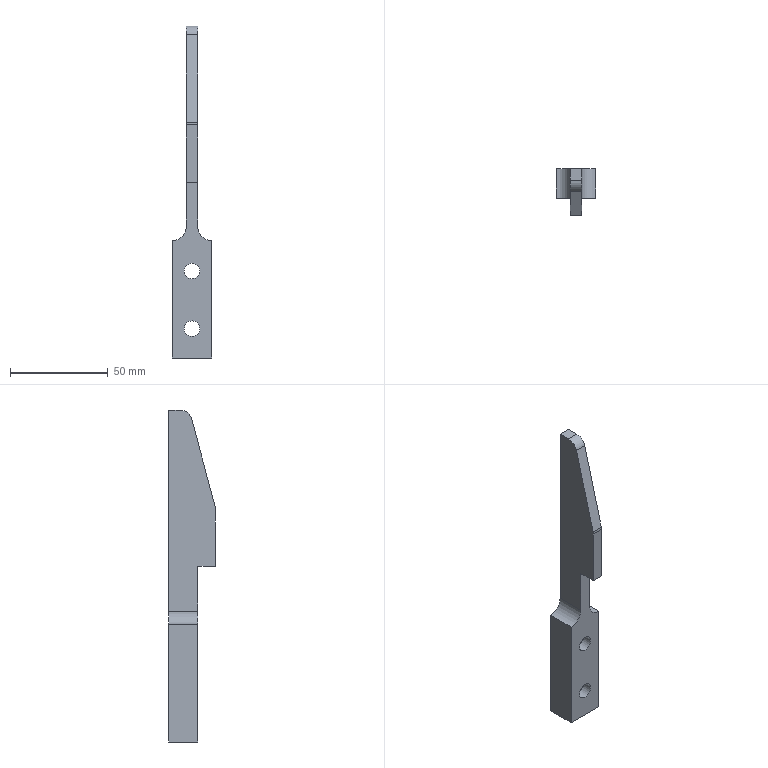Part | NX | features solid 2 | 1 solid | 21 faces | box 20 x 24 x 170 mm | volume 26920 mm3 | plane 13 | cylinder 8 | commonest cylinder face diameters 14 x4 8 x2 10 x1 12 x1
STEP:
#1=CARTESIAN_POINT('',(-125.,490.,-140.));
#2=VERTEX_POINT('',#1);
#3=CARTESIAN_POINT('',(-125.,490.,-80.));
#4=VERTEX_POINT('',#3);
#5=CARTESIAN_POINT('',(-125.,490.,-110.));
#6=DIRECTION('',(0.,0.,1.));
#7=VECTOR('',#6,1000.);
#8=LINE('',#5,#7);
#9=EDGE_CURVE('',#2,#4,#8,.T.);
#10=ORIENTED_EDGE('',*,*,#9,.F.);
#11=CARTESIAN_POINT('',(-125.,505.,-140.));
#12=VERTEX_POINT('',#11);
#13=CARTESIAN_POINT('',(-125.,490.,-140.));
#14=DIRECTION('',(0.,1.,0.));
#15=VECTOR('',#14,1000.);
#16=LINE('',#13,#15);
#17=EDGE_CURVE('',#2,#12,#16,.T.);
#18=ORIENTED_EDGE('',*,*,#17,.T.);
#19=CARTESIAN_POINT('',(-125.,505.,-80.));
#20=VERTEX_POINT('',#19);
#21=CARTESIAN_POINT('',(-125.,505.,-110.));
#22=DIRECTION('',(0.,0.,1.));
#23=VECTOR('',#22,1000.);
#24=LINE('',#21,#23);
#25=EDGE_CURVE('',#12,#20,#24,.T.);
#26=ORIENTED_EDGE('',*,*,#25,.T.);
#27=CARTESIAN_POINT('',(-125.,490.,-80.));
#28=DIRECTION('',(0.,1.,0.));
#29=VECTOR('',#28,1000.);
#30=LINE('',#27,#29);
#31=EDGE_CURVE('',#4,#20,#30,.T.);
#32=ORIENTED_EDGE('',*,*,#31,.F.);
#33=EDGE_LOOP('',(#10,#18,#26,#32));
#34=FACE_BOUND('',#33,.T.);
#35=CARTESIAN_POINT('',(-125.,490.,-110.));
#36=DIRECTION('',(1.,0.,0.));
#37=DIRECTION('',(0.,1.,0.));
#38=AXIS2_PLACEMENT_3D('',#35,#36,#37);
#39=PLANE('',#38);
#40=ADVANCED_FACE('',(#34),#39,.T.);
#41=CARTESIAN_POINT('',(-135.,505.,-118.));
#42=VERTEX_POINT('',#41);
#43=CARTESIAN_POINT('',(-135.,505.,-125.));
#44=DIRECTION('',(0.,-1.,0.));
#45=DIRECTION('',(0.,0.,1.));
#46=AXIS2_PLACEMENT_3D('',#43,#44,#45);
#47=CIRCLE('',#46,7.);
#48=EDGE_CURVE('',#42,#42,#47,.T.);
#49=ORIENTED_EDGE('',*,*,#48,.T.);
#50=EDGE_LOOP('',(#49));
#51=FACE_BOUND('',#50,.T.);
#52=CARTESIAN_POINT('',(-135.,505.,-102.5));
#53=VERTEX_POINT('',#52);
#54=CARTESIAN_POINT('',(-135.,505.,-95.5));
#55=DIRECTION('',(0.,1.,0.));
#56=DIRECTION('',(0.,0.,-1.));
#57=AXIS2_PLACEMENT_3D('',#54,#55,#56);
#58=CIRCLE('',#57,7.);
#59=EDGE_CURVE('',#53,#53,#58,.F.);
#60=ORIENTED_EDGE('',*,*,#59,.T.);
#61=EDGE_LOOP('',(#60));
#62=FACE_BOUND('',#61,.T.);
#63=ORIENTED_EDGE('',*,*,#25,.F.);
#64=CARTESIAN_POINT('',(-145.,505.,-140.));
#65=VERTEX_POINT('',#64);
#66=CARTESIAN_POINT('',(-125.,505.,-140.));
#67=DIRECTION('',(-1.,0.,0.));
#68=VECTOR('',#67,1000.);
#69=LINE('',#66,#68);
#70=EDGE_CURVE('',#12,#65,#69,.T.);
#71=ORIENTED_EDGE('',*,*,#70,.T.);
#72=CARTESIAN_POINT('',(-145.,505.,-80.));
#73=VERTEX_POINT('',#72);
#74=CARTESIAN_POINT('',(-145.,505.,-110.));
#75=DIRECTION('',(0.,0.,1.));
#76=VECTOR('',#75,1000.);
#77=LINE('',#74,#76);
#78=EDGE_CURVE('',#65,#73,#77,.T.);
#79=ORIENTED_EDGE('',*,*,#78,.T.);
#80=CARTESIAN_POINT('',(-138.,505.,-73.));
#81=VERTEX_POINT('',#80);
#82=CARTESIAN_POINT('',(-145.,505.,-73.));
#83=DIRECTION('',(0.,1.,0.));
#84=DIRECTION('',(0.,0.,-1.));
#85=AXIS2_PLACEMENT_3D('',#82,#83,#84);
#86=CIRCLE('',#85,7.);
#87=EDGE_CURVE('',#73,#81,#86,.F.);
#88=ORIENTED_EDGE('',*,*,#87,.T.);
#89=CARTESIAN_POINT('',(-138.,505.,30.));
#90=VERTEX_POINT('',#89);
#91=CARTESIAN_POINT('',(-138.,505.,-50.));
#92=DIRECTION('',(0.,0.,1.));
#93=VECTOR('',#92,1000.);
#94=LINE('',#91,#93);
#95=EDGE_CURVE('',#81,#90,#94,.T.);
#96=ORIENTED_EDGE('',*,*,#95,.T.);
#97=CARTESIAN_POINT('',(-132.,505.,30.));
#98=VERTEX_POINT('',#97);
#99=CARTESIAN_POINT('',(-132.,505.,30.));
#100=DIRECTION('',(-1.,0.,0.));
#101=VECTOR('',#100,1000.);
#102=LINE('',#99,#101);
#103=EDGE_CURVE('',#98,#90,#102,.T.);
#104=ORIENTED_EDGE('',*,*,#103,.F.);
#105=CARTESIAN_POINT('',(-132.,505.,-73.));
#106=VERTEX_POINT('',#105);
#107=CARTESIAN_POINT('',(-132.,505.,-50.));
#108=DIRECTION('',(0.,0.,1.));
#109=VECTOR('',#108,1000.);
#110=LINE('',#107,#109);
#111=EDGE_CURVE('',#106,#98,#110,.T.);
#112=ORIENTED_EDGE('',*,*,#111,.F.);
#113=CARTESIAN_POINT('',(-125.,505.,-73.));
#114=DIRECTION('',(0.,1.,0.));
#115=DIRECTION('',(0.,0.,-1.));
#116=AXIS2_PLACEMENT_3D('',#113,#114,#115);
#117=CIRCLE('',#116,7.);
#118=EDGE_CURVE('',#106,#20,#117,.F.);
#119=ORIENTED_EDGE('',*,*,#118,.T.);
#120=EDGE_LOOP('',(#63,#71,#79,#88,#96,#104,#112,#119));
#121=FACE_BOUND('',#120,.T.);
#122=CARTESIAN_POINT('',(-125.,505.,-110.));
#123=DIRECTION('',(0.,1.,0.));
#124=DIRECTION('',(-1.,0.,0.));
#125=AXIS2_PLACEMENT_3D('',#122,#123,#124);
#126=PLANE('',#125);
#127=ADVANCED_FACE('',(#51,#62,#121),#126,.T.);
#128=ORIENTED_EDGE('',*,*,#78,.F.);
#129=CARTESIAN_POINT('',(-145.,490.,-140.));
#130=VERTEX_POINT('',#129);
#131=CARTESIAN_POINT('',(-145.,490.,-140.));
#132=DIRECTION('',(0.,1.,0.));
#133=VECTOR('',#132,1000.);
#134=LINE('',#131,#133);
#135=EDGE_CURVE('',#130,#65,#134,.T.);
#136=ORIENTED_EDGE('',*,*,#135,.F.);
#137=CARTESIAN_POINT('',(-145.,490.,-80.));
#138=VERTEX_POINT('',#137);
#139=CARTESIAN_POINT('',(-145.,490.,-110.));
#140=DIRECTION('',(0.,0.,1.));
#141=VECTOR('',#140,1000.);
#142=LINE('',#139,#141);
#143=EDGE_CURVE('',#130,#138,#142,.T.);
#144=ORIENTED_EDGE('',*,*,#143,.T.);
#145=CARTESIAN_POINT('',(-145.,490.,-80.));
#146=DIRECTION('',(0.,1.,0.));
#147=VECTOR('',#146,1000.);
#148=LINE('',#145,#147);
#149=EDGE_CURVE('',#138,#73,#148,.T.);
#150=ORIENTED_EDGE('',*,*,#149,.T.);
#151=EDGE_LOOP('',(#128,#136,#144,#150));
#152=FACE_BOUND('',#151,.T.);
#153=CARTESIAN_POINT('',(-145.,490.,-110.));
#154=DIRECTION('',(1.,0.,0.));
#155=DIRECTION('',(0.,1.,0.));
#156=AXIS2_PLACEMENT_3D('',#153,#154,#155);
#157=PLANE('',#156);
#158=ADVANCED_FACE('',(#152),#157,.F.);
#159=CARTESIAN_POINT('',(-135.,490.,-99.5));
#160=VERTEX_POINT('',#159);
#161=CARTESIAN_POINT('',(-135.,490.,-95.5));
#162=DIRECTION('',(0.,1.,0.));
#163=DIRECTION('',(0.,0.,-1.));
#164=AXIS2_PLACEMENT_3D('',#161,#162,#163);
#165=CIRCLE('',#164,4.);
#166=EDGE_CURVE('',#160,#160,#165,.T.);
#167=ORIENTED_EDGE('',*,*,#166,.T.);
#168=EDGE_LOOP('',(#167));
#169=FACE_BOUND('',#168,.T.);
#170=CARTESIAN_POINT('',(-135.,490.,-129.));
#171=VERTEX_POINT('',#170);
#172=CARTESIAN_POINT('',(-135.,490.,-125.));
#173=DIRECTION('',(0.,1.,0.));
#174=DIRECTION('',(0.,0.,-1.));
#175=AXIS2_PLACEMENT_3D('',#172,#173,#174);
#176=CIRCLE('',#175,4.);
#177=EDGE_CURVE('',#171,#171,#176,.T.);
#178=ORIENTED_EDGE('',*,*,#177,.T.);
#179=EDGE_LOOP('',(#178));
#180=FACE_BOUND('',#179,.T.);
#181=CARTESIAN_POINT('',(-132.,490.,-50.));
#182=VERTEX_POINT('',#181);
#183=CARTESIAN_POINT('',(-132.,490.,-73.));
#184=VERTEX_POINT('',#183);
#185=CARTESIAN_POINT('',(-132.,490.,-43.));
#186=DIRECTION('',(0.,0.,1.));
#187=VECTOR('',#186,1000.);
#188=LINE('',#185,#187);
#189=EDGE_CURVE('',#182,#184,#188,.F.);
#190=ORIENTED_EDGE('',*,*,#189,.F.);
#191=CARTESIAN_POINT('',(-138.,490.,-50.));
#192=VERTEX_POINT('',#191);
#193=CARTESIAN_POINT('',(-132.,490.,-50.));
#194=DIRECTION('',(1.,0.,0.));
#195=VECTOR('',#194,1000.);
#196=LINE('',#193,#195);
#197=EDGE_CURVE('',#182,#192,#196,.F.);
#198=ORIENTED_EDGE('',*,*,#197,.T.);
#199=CARTESIAN_POINT('',(-138.,490.,-73.));
#200=VERTEX_POINT('',#199);
#201=CARTESIAN_POINT('',(-138.,490.,-43.));
#202=DIRECTION('',(0.,0.,-1.));
#203=VECTOR('',#202,1000.);
#204=LINE('',#201,#203);
#205=EDGE_CURVE('',#192,#200,#204,.T.);
#206=ORIENTED_EDGE('',*,*,#205,.T.);
#207=CARTESIAN_POINT('',(-145.,490.,-73.));
#208=DIRECTION('',(0.,1.,0.));
#209=DIRECTION('',(0.,0.,-1.));
#210=AXIS2_PLACEMENT_3D('',#207,#208,#209);
#211=CIRCLE('',#210,7.);
#212=EDGE_CURVE('',#200,#138,#211,.T.);
#213=ORIENTED_EDGE('',*,*,#212,.T.);
#214=ORIENTED_EDGE('',*,*,#143,.F.);
#215=CARTESIAN_POINT('',(-125.,490.,-140.));
#216=DIRECTION('',(-1.,0.,0.));
#217=VECTOR('',#216,1000.);
#218=LINE('',#215,#217);
#219=EDGE_CURVE('',#2,#130,#218,.T.);
#220=ORIENTED_EDGE('',*,*,#219,.F.);
#221=ORIENTED_EDGE('',*,*,#9,.T.);
#222=CARTESIAN_POINT('',(-125.,490.,-73.));
#223=DIRECTION('',(0.,1.,0.));
#224=DIRECTION('',(0.,0.,-1.));
#225=AXIS2_PLACEMENT_3D('',#222,#223,#224);
#226=CIRCLE('',#225,7.);
#227=EDGE_CURVE('',#4,#184,#226,.T.);
#228=ORIENTED_EDGE('',*,*,#227,.T.);
#229=EDGE_LOOP('',(#190,#198,#206,#213,#214,#220,#221,#228));
#230=FACE_BOUND('',#229,.T.);
#231=CARTESIAN_POINT('',(-125.,490.,-110.));
#232=DIRECTION('',(0.,1.,0.));
#233=DIRECTION('',(-1.,0.,0.));
#234=AXIS2_PLACEMENT_3D('',#231,#232,#233);
#235=PLANE('',#234);
#236=ADVANCED_FACE('',(#169,#180,#230),#235,.F.);
#237=ORIENTED_EDGE('',*,*,#135,.T.);
#238=ORIENTED_EDGE('',*,*,#70,.F.);
#239=ORIENTED_EDGE('',*,*,#17,.F.);
#240=ORIENTED_EDGE('',*,*,#219,.T.);
#241=EDGE_LOOP('',(#237,#238,#239,#240));
#242=FACE_BOUND('',#241,.T.);
#243=CARTESIAN_POINT('',(-125.,490.,-140.));
#244=DIRECTION('',(0.,0.,1.));
#245=DIRECTION('',(0.,1.,0.));
#246=AXIS2_PLACEMENT_3D('',#243,#244,#245);
#247=PLANE('',#246);
#248=ADVANCED_FACE('',(#242),#247,.F.);
#249=CARTESIAN_POINT('',(-132.,493.206,25.553));
#250=VERTEX_POINT('',#249);
#251=CARTESIAN_POINT('',(-132.,481.17,-19.364));
#252=VERTEX_POINT('',#251);
#253=CARTESIAN_POINT('',(-132.,478.398,-29.711));
#254=DIRECTION('',(0.,-0.2588,-0.9659));
#255=VECTOR('',#254,1000.);
#256=LINE('',#253,#255);
#257=EDGE_CURVE('',#250,#252,#256,.T.);
#258=ORIENTED_EDGE('',*,*,#257,.T.);
#259=CARTESIAN_POINT('',(-132.,481.,-20.658));
#260=VERTEX_POINT('',#259);
#261=CARTESIAN_POINT('',(-132.,486.,-20.658));
#262=DIRECTION('',(1.,0.,0.));
#263=DIRECTION('',(0.,0.,-1.));
#264=AXIS2_PLACEMENT_3D('',#261,#262,#263);
#265=CIRCLE('',#264,5.);
#266=EDGE_CURVE('',#252,#260,#265,.T.);
#267=ORIENTED_EDGE('',*,*,#266,.T.);
#268=CARTESIAN_POINT('',(-132.,481.,-50.));
#269=VERTEX_POINT('',#268);
#270=CARTESIAN_POINT('',(-132.,481.,-43.));
#271=DIRECTION('',(0.,0.,1.));
#272=VECTOR('',#271,1000.);
#273=LINE('',#270,#272);
#274=EDGE_CURVE('',#269,#260,#273,.T.);
#275=ORIENTED_EDGE('',*,*,#274,.F.);
#276=CARTESIAN_POINT('',(-132.,490.,-50.));
#277=DIRECTION('',(0.,1.,0.));
#278=VECTOR('',#277,1000.);
#279=LINE('',#276,#278);
#280=EDGE_CURVE('',#182,#269,#279,.F.);
#281=ORIENTED_EDGE('',*,*,#280,.F.);
#282=ORIENTED_EDGE('',*,*,#189,.T.);
#283=CARTESIAN_POINT('',(-132.,505.,-73.));
#284=DIRECTION('',(0.,1.,0.));
#285=VECTOR('',#284,1000.);
#286=LINE('',#283,#285);
#287=EDGE_CURVE('',#184,#106,#286,.T.);
#288=ORIENTED_EDGE('',*,*,#287,.T.);
#289=ORIENTED_EDGE('',*,*,#111,.T.);
#290=CARTESIAN_POINT('',(-132.,499.001,30.));
#291=VERTEX_POINT('',#290);
#292=CARTESIAN_POINT('',(-132.,490.,30.));
#293=DIRECTION('',(0.,1.,0.));
#294=VECTOR('',#293,1000.);
#295=LINE('',#292,#294);
#296=EDGE_CURVE('',#291,#98,#295,.T.);
#297=ORIENTED_EDGE('',*,*,#296,.F.);
#298=CARTESIAN_POINT('',(-132.,499.001,24.));
#299=DIRECTION('',(1.,0.,0.));
#300=DIRECTION('',(0.,0.,-1.));
#301=AXIS2_PLACEMENT_3D('',#298,#299,#300);
#302=CIRCLE('',#301,6.);
#303=EDGE_CURVE('',#291,#250,#302,.T.);
#304=ORIENTED_EDGE('',*,*,#303,.T.);
#305=EDGE_LOOP('',(#258,#267,#275,#281,#282,#288,#289,#297,#304));
#306=FACE_BOUND('',#305,.T.);
#307=CARTESIAN_POINT('',(-132.,490.,-50.));
#308=DIRECTION('',(1.,0.,0.));
#309=DIRECTION('',(0.,1.,0.));
#310=AXIS2_PLACEMENT_3D('',#307,#308,#309);
#311=PLANE('',#310);
#312=ADVANCED_FACE('',(#306),#311,.T.);
#313=CARTESIAN_POINT('',(-138.,481.,-50.));
#314=VERTEX_POINT('',#313);
#315=CARTESIAN_POINT('',(-138.,481.,-20.658));
#316=VERTEX_POINT('',#315);
#317=CARTESIAN_POINT('',(-138.,481.,-43.));
#318=DIRECTION('',(0.,0.,-1.));
#319=VECTOR('',#318,1000.);
#320=LINE('',#317,#319);
#321=EDGE_CURVE('',#314,#316,#320,.F.);
#322=ORIENTED_EDGE('',*,*,#321,.T.);
#323=CARTESIAN_POINT('',(-138.,481.17,-19.364));
#324=VERTEX_POINT('',#323);
#325=CARTESIAN_POINT('',(-138.,486.,-20.658));
#326=DIRECTION('',(1.,0.,0.));
#327=DIRECTION('',(0.,0.,-1.));
#328=AXIS2_PLACEMENT_3D('',#325,#326,#327);
#329=CIRCLE('',#328,5.);
#330=EDGE_CURVE('',#316,#324,#329,.F.);
#331=ORIENTED_EDGE('',*,*,#330,.T.);
#332=CARTESIAN_POINT('',(-138.,493.206,25.553));
#333=VERTEX_POINT('',#332);
#334=CARTESIAN_POINT('',(-138.,478.398,-29.711));
#335=DIRECTION('',(0.,-0.2588,-0.9659));
#336=VECTOR('',#335,1000.);
#337=LINE('',#334,#336);
#338=EDGE_CURVE('',#324,#333,#337,.F.);
#339=ORIENTED_EDGE('',*,*,#338,.T.);
#340=CARTESIAN_POINT('',(-138.,499.001,30.));
#341=VERTEX_POINT('',#340);
#342=CARTESIAN_POINT('',(-138.,499.001,24.));
#343=DIRECTION('',(1.,0.,0.));
#344=DIRECTION('',(0.,0.,-1.));
#345=AXIS2_PLACEMENT_3D('',#342,#343,#344);
#346=CIRCLE('',#345,6.);
#347=EDGE_CURVE('',#333,#341,#346,.F.);
#348=ORIENTED_EDGE('',*,*,#347,.T.);
#349=CARTESIAN_POINT('',(-138.,490.,30.));
#350=DIRECTION('',(0.,-1.,0.));
#351=VECTOR('',#350,1000.);
#352=LINE('',#349,#351);
#353=EDGE_CURVE('',#341,#90,#352,.F.);
#354=ORIENTED_EDGE('',*,*,#353,.T.);
#355=ORIENTED_EDGE('',*,*,#95,.F.);
#356=CARTESIAN_POINT('',(-138.,490.,-73.));
#357=DIRECTION('',(0.,1.,0.));
#358=VECTOR('',#357,1000.);
#359=LINE('',#356,#358);
#360=EDGE_CURVE('',#81,#200,#359,.F.);
#361=ORIENTED_EDGE('',*,*,#360,.T.);
#362=ORIENTED_EDGE('',*,*,#205,.F.);
#363=CARTESIAN_POINT('',(-138.,490.,-50.));
#364=DIRECTION('',(0.,1.,0.));
#365=VECTOR('',#364,1000.);
#366=LINE('',#363,#365);
#367=EDGE_CURVE('',#192,#314,#366,.F.);
#368=ORIENTED_EDGE('',*,*,#367,.T.);
#369=EDGE_LOOP('',(#322,#331,#339,#348,#354,#355,#361,#362,#368));
#370=FACE_BOUND('',#369,.T.);
#371=CARTESIAN_POINT('',(-138.,490.,-50.));
#372=DIRECTION('',(1.,0.,0.));
#373=DIRECTION('',(0.,1.,0.));
#374=AXIS2_PLACEMENT_3D('',#371,#372,#373);
#375=PLANE('',#374);
#376=ADVANCED_FACE('',(#370),#375,.F.);
#377=ORIENTED_EDGE('',*,*,#353,.F.);
#378=CARTESIAN_POINT('',(-132.,499.001,30.));
#379=DIRECTION('',(-1.,0.,0.));
#380=VECTOR('',#379,1000.);
#381=LINE('',#378,#380);
#382=EDGE_CURVE('',#341,#291,#381,.F.);
#383=ORIENTED_EDGE('',*,*,#382,.T.);
#384=ORIENTED_EDGE('',*,*,#296,.T.);
#385=ORIENTED_EDGE('',*,*,#103,.T.);
#386=EDGE_LOOP('',(#377,#383,#384,#385));
#387=FACE_BOUND('',#386,.T.);
#388=CARTESIAN_POINT('',(-132.,490.,30.));
#389=DIRECTION('',(0.,0.,1.));
#390=DIRECTION('',(0.,1.,0.));
#391=AXIS2_PLACEMENT_3D('',#388,#389,#390);
#392=PLANE('',#391);
#393=ADVANCED_FACE('',(#387),#392,.T.);
#394=ORIENTED_EDGE('',*,*,#212,.F.);
#395=ORIENTED_EDGE('',*,*,#360,.F.);
#396=ORIENTED_EDGE('',*,*,#87,.F.);
#397=ORIENTED_EDGE('',*,*,#149,.F.);
#398=EDGE_LOOP('',(#394,#395,#396,#397));
#399=FACE_BOUND('',#398,.T.);
#400=CARTESIAN_POINT('',(-145.,490.,-73.));
#401=DIRECTION('',(0.,1.,0.));
#402=DIRECTION('',(0.,0.,-1.));
#403=AXIS2_PLACEMENT_3D('',#400,#401,#402);
#404=CYLINDRICAL_SURFACE('',#403,7.);
#405=ADVANCED_FACE('',(#399),#404,.F.);
#406=ORIENTED_EDGE('',*,*,#227,.F.);
#407=ORIENTED_EDGE('',*,*,#31,.T.);
#408=ORIENTED_EDGE('',*,*,#118,.F.);
#409=ORIENTED_EDGE('',*,*,#287,.F.);
#410=EDGE_LOOP('',(#406,#407,#408,#409));
#411=FACE_BOUND('',#410,.T.);
#412=CARTESIAN_POINT('',(-125.,490.,-73.));
#413=DIRECTION('',(0.,-1.,0.));
#414=DIRECTION('',(0.,0.,1.));
#415=AXIS2_PLACEMENT_3D('',#412,#413,#414);
#416=CYLINDRICAL_SURFACE('',#415,7.);
#417=ADVANCED_FACE('',(#411),#416,.F.);
#418=ORIENTED_EDGE('',*,*,#197,.F.);
#419=ORIENTED_EDGE('',*,*,#280,.T.);
#420=CARTESIAN_POINT('',(-132.,481.,-50.));
#421=DIRECTION('',(-1.,0.,0.));
#422=VECTOR('',#421,1000.);
#423=LINE('',#420,#422);
#424=EDGE_CURVE('',#269,#314,#423,.T.);
#425=ORIENTED_EDGE('',*,*,#424,.T.);
#426=ORIENTED_EDGE('',*,*,#367,.F.);
#427=EDGE_LOOP('',(#418,#419,#425,#426));
#428=FACE_BOUND('',#427,.T.);
#429=CARTESIAN_POINT('',(-132.,490.,-50.));
#430=DIRECTION('',(0.,0.,1.));
#431=DIRECTION('',(0.,-1.,0.));
#432=AXIS2_PLACEMENT_3D('',#429,#430,#431);
#433=PLANE('',#432);
#434=ADVANCED_FACE('',(#428),#433,.F.);
#435=ORIENTED_EDGE('',*,*,#274,.T.);
#436=CARTESIAN_POINT('',(-132.,481.,-20.658));
#437=DIRECTION('',(-1.,0.,0.));
#438=VECTOR('',#437,1000.);
#439=LINE('',#436,#438);
#440=EDGE_CURVE('',#260,#316,#439,.T.);
#441=ORIENTED_EDGE('',*,*,#440,.T.);
#442=ORIENTED_EDGE('',*,*,#321,.F.);
#443=ORIENTED_EDGE('',*,*,#424,.F.);
#444=EDGE_LOOP('',(#435,#441,#442,#443));
#445=FACE_BOUND('',#444,.T.);
#446=CARTESIAN_POINT('',(-132.,481.,-43.));
#447=DIRECTION('',(0.,1.,0.));
#448=DIRECTION('',(0.,0.,1.));
#449=AXIS2_PLACEMENT_3D('',#446,#447,#448);
#450=PLANE('',#449);
#451=ADVANCED_FACE('',(#445),#450,.F.);
#452=ORIENTED_EDGE('',*,*,#338,.F.);
#453=CARTESIAN_POINT('',(-132.,481.17,-19.364));
#454=DIRECTION('',(1.,0.,0.));
#455=VECTOR('',#454,1000.);
#456=LINE('',#453,#455);
#457=EDGE_CURVE('',#324,#252,#456,.T.);
#458=ORIENTED_EDGE('',*,*,#457,.T.);
#459=ORIENTED_EDGE('',*,*,#257,.F.);
#460=CARTESIAN_POINT('',(-132.,493.206,25.553));
#461=DIRECTION('',(-1.,0.,0.));
#462=VECTOR('',#461,1000.);
#463=LINE('',#460,#462);
#464=EDGE_CURVE('',#250,#333,#463,.T.);
#465=ORIENTED_EDGE('',*,*,#464,.T.);
#466=EDGE_LOOP('',(#452,#458,#459,#465));
#467=FACE_BOUND('',#466,.T.);
#468=CARTESIAN_POINT('',(-132.,493.295,25.886));
#469=DIRECTION('',(0.,-0.9659,0.2588));
#470=DIRECTION('',(0.,0.2588,0.9659));
#471=AXIS2_PLACEMENT_3D('',#468,#469,#470);
#472=PLANE('',#471);
#473=ADVANCED_FACE('',(#467),#472,.T.);
#474=CARTESIAN_POINT('',(-135.,495.,-121.));
#475=VERTEX_POINT('',#474);
#476=CARTESIAN_POINT('',(-135.,495.,-125.));
#477=DIRECTION('',(0.,-1.,0.));
#478=DIRECTION('',(0.,0.,1.));
#479=AXIS2_PLACEMENT_3D('',#476,#477,#478);
#480=CIRCLE('',#479,4.);
#481=EDGE_CURVE('',#475,#475,#480,.F.);
#482=ORIENTED_EDGE('',*,*,#481,.T.);
#483=EDGE_LOOP('',(#482));
#484=FACE_BOUND('',#483,.T.);
#485=ORIENTED_EDGE('',*,*,#177,.F.);
#486=EDGE_LOOP('',(#485));
#487=FACE_BOUND('',#486,.T.);
#488=CARTESIAN_POINT('',(-135.,490.,-125.));
#489=DIRECTION('',(0.,1.,0.));
#490=DIRECTION('',(0.,0.,-1.));
#491=AXIS2_PLACEMENT_3D('',#488,#489,#490);
#492=CYLINDRICAL_SURFACE('',#491,4.);
#493=ADVANCED_FACE('',(#484,#487),#492,.F.);
#494=CARTESIAN_POINT('',(-135.,495.,-91.5));
#495=VERTEX_POINT('',#494);
#496=CARTESIAN_POINT('',(-135.,495.,-95.5));
#497=DIRECTION('',(0.,-1.,0.));
#498=DIRECTION('',(0.,0.,1.));
#499=AXIS2_PLACEMENT_3D('',#496,#497,#498);
#500=CIRCLE('',#499,4.);
#501=EDGE_CURVE('',#495,#495,#500,.F.);
#502=ORIENTED_EDGE('',*,*,#501,.T.);
#503=EDGE_LOOP('',(#502));
#504=FACE_BOUND('',#503,.T.);
#505=ORIENTED_EDGE('',*,*,#166,.F.);
#506=EDGE_LOOP('',(#505));
#507=FACE_BOUND('',#506,.T.);
#508=CARTESIAN_POINT('',(-135.,490.,-95.5));
#509=DIRECTION('',(0.,1.,0.));
#510=DIRECTION('',(0.,0.,-1.));
#511=AXIS2_PLACEMENT_3D('',#508,#509,#510);
#512=CYLINDRICAL_SURFACE('',#511,4.);
#513=ADVANCED_FACE('',(#504,#507),#512,.F.);
#514=CARTESIAN_POINT('',(-135.,495.,-88.5));
#515=VERTEX_POINT('',#514);
#516=CARTESIAN_POINT('',(-135.,495.,-95.5));
#517=DIRECTION('',(0.,-1.,0.));
#518=DIRECTION('',(0.,0.,1.));
#519=AXIS2_PLACEMENT_3D('',#516,#517,#518);
#520=CIRCLE('',#519,7.);
#521=EDGE_CURVE('',#515,#515,#520,.T.);
#522=ORIENTED_EDGE('',*,*,#521,.F.);
#523=EDGE_LOOP('',(#522));
#524=FACE_BOUND('',#523,.T.);
#525=ORIENTED_EDGE('',*,*,#501,.F.);
#526=EDGE_LOOP('',(#525));
#527=FACE_BOUND('',#526,.T.);
#528=CARTESIAN_POINT('',(-135.,495.,-65.5));
#529=DIRECTION('',(0.,-1.,0.));
#530=DIRECTION('',(0.,0.,1.));
#531=AXIS2_PLACEMENT_3D('',#528,#529,#530);
#532=PLANE('',#531);
#533=ADVANCED_FACE('',(#524,#527),#532,.F.);
#534=ORIENTED_EDGE('',*,*,#521,.T.);
#535=EDGE_LOOP('',(#534));
#536=FACE_BOUND('',#535,.T.);
#537=ORIENTED_EDGE('',*,*,#59,.F.);
#538=EDGE_LOOP('',(#537));
#539=FACE_BOUND('',#538,.T.);
#540=CARTESIAN_POINT('',(-135.,505.,-95.5));
#541=DIRECTION('',(0.,-1.,0.));
#542=DIRECTION('',(0.,0.,1.));
#543=AXIS2_PLACEMENT_3D('',#540,#541,#542);
#544=CYLINDRICAL_SURFACE('',#543,7.);
#545=ADVANCED_FACE('',(#536,#539),#544,.F.);
#546=CARTESIAN_POINT('',(-135.,495.,-118.));
#547=VERTEX_POINT('',#546);
#548=CARTESIAN_POINT('',(-135.,495.,-125.));
#549=DIRECTION('',(0.,-1.,0.));
#550=DIRECTION('',(0.,0.,1.));
#551=AXIS2_PLACEMENT_3D('',#548,#549,#550);
#552=CIRCLE('',#551,7.);
#553=EDGE_CURVE('',#547,#547,#552,.T.);
#554=ORIENTED_EDGE('',*,*,#553,.F.);
#555=EDGE_LOOP('',(#554));
#556=FACE_BOUND('',#555,.T.);
#557=ORIENTED_EDGE('',*,*,#481,.F.);
#558=EDGE_LOOP('',(#557));
#559=FACE_BOUND('',#558,.T.);
#560=CARTESIAN_POINT('',(-135.,495.,-95.));
#561=DIRECTION('',(0.,-1.,0.));
#562=DIRECTION('',(0.,0.,1.));
#563=AXIS2_PLACEMENT_3D('',#560,#561,#562);
#564=PLANE('',#563);
#565=ADVANCED_FACE('',(#556,#559),#564,.F.);
#566=ORIENTED_EDGE('',*,*,#553,.T.);
#567=EDGE_LOOP('',(#566));
#568=FACE_BOUND('',#567,.T.);
#569=ORIENTED_EDGE('',*,*,#48,.F.);
#570=EDGE_LOOP('',(#569));
#571=FACE_BOUND('',#570,.T.);
#572=CARTESIAN_POINT('',(-135.,505.,-125.));
#573=DIRECTION('',(0.,-1.,0.));
#574=DIRECTION('',(0.,0.,1.));
#575=AXIS2_PLACEMENT_3D('',#572,#573,#574);
#576=CYLINDRICAL_SURFACE('',#575,7.);
#577=ADVANCED_FACE('',(#568,#571),#576,.F.);
#578=ORIENTED_EDGE('',*,*,#303,.F.);
#579=ORIENTED_EDGE('',*,*,#382,.F.);
#580=ORIENTED_EDGE('',*,*,#347,.F.);
#581=ORIENTED_EDGE('',*,*,#464,.F.);
#582=EDGE_LOOP('',(#578,#579,#580,#581));
#583=FACE_BOUND('',#582,.T.);
#584=CARTESIAN_POINT('',(-132.,499.001,24.));
#585=DIRECTION('',(-1.,0.,0.));
#586=DIRECTION('',(0.,0.,1.));
#587=AXIS2_PLACEMENT_3D('',#584,#585,#586);
#588=CYLINDRICAL_SURFACE('',#587,6.);
#589=ADVANCED_FACE('',(#583),#588,.T.);
#590=ORIENTED_EDGE('',*,*,#266,.F.);
#591=ORIENTED_EDGE('',*,*,#457,.F.);
#592=ORIENTED_EDGE('',*,*,#330,.F.);
#593=ORIENTED_EDGE('',*,*,#440,.F.);
#594=EDGE_LOOP('',(#590,#591,#592,#593));
#595=FACE_BOUND('',#594,.T.);
#596=CARTESIAN_POINT('',(-132.,486.,-20.658));
#597=DIRECTION('',(1.,0.,0.));
#598=DIRECTION('',(0.,0.,-1.));
#599=AXIS2_PLACEMENT_3D('',#596,#597,#598);
#600=CYLINDRICAL_SURFACE('',#599,5.);
#601=ADVANCED_FACE('',(#595),#600,.T.);
#602=CLOSED_SHELL('',(#40,#127,#158,#236,#248,#312,#376,#393,#405,#417,#434,#451,#473,#493,#513,#533,#545,#565,#577,#589,#601));
#603=MANIFOLD_SOLID_BREP('',#602);
#604=(LENGTH_UNIT()NAMED_UNIT(*)SI_UNIT(.MILLI.,.METRE.));
#605=UNCERTAINTY_MEASURE_WITH_UNIT(LENGTH_MEASURE(0.00001),#604,'','');
#606=(NAMED_UNIT(*)PLANE_ANGLE_UNIT()SI_UNIT($,.RADIAN.));
#607=(NAMED_UNIT(*)SI_UNIT($,.STERADIAN.)SOLID_ANGLE_UNIT());
#608=(GEOMETRIC_REPRESENTATION_CONTEXT(3)GLOBAL_UNCERTAINTY_ASSIGNED_CONTEXT((#605))GLOBAL_UNIT_ASSIGNED_CONTEXT((#604,#606,#607))REPRESENTATION_CONTEXT('',''));
#609=ADVANCED_BREP_SHAPE_REPRESENTATION('',(#603),#608);